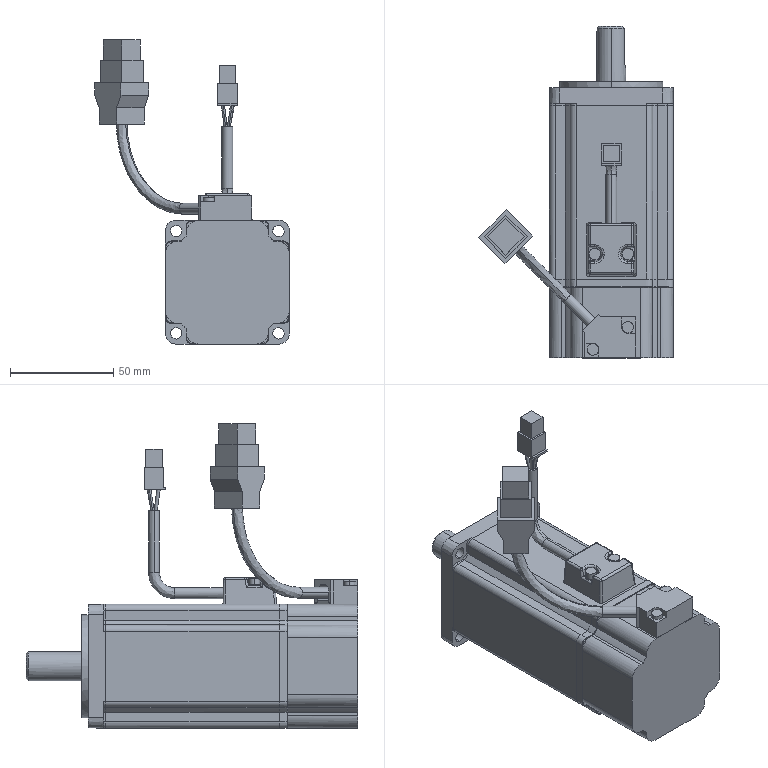Part | STEP file | Delta 400W servo motor ECMA-CX0604ES | 1 solid | 1986 faces | box 94.241 x 160.702 x 147.367 mm | volume 450484 mm3 | plane 1259 | spline 540 | cylinder 163 | cone 24 | commonest cylinder face diameters 6 x41 2 x20 5.5 x16 0.6 x12 1.5 x11 5.3 x8